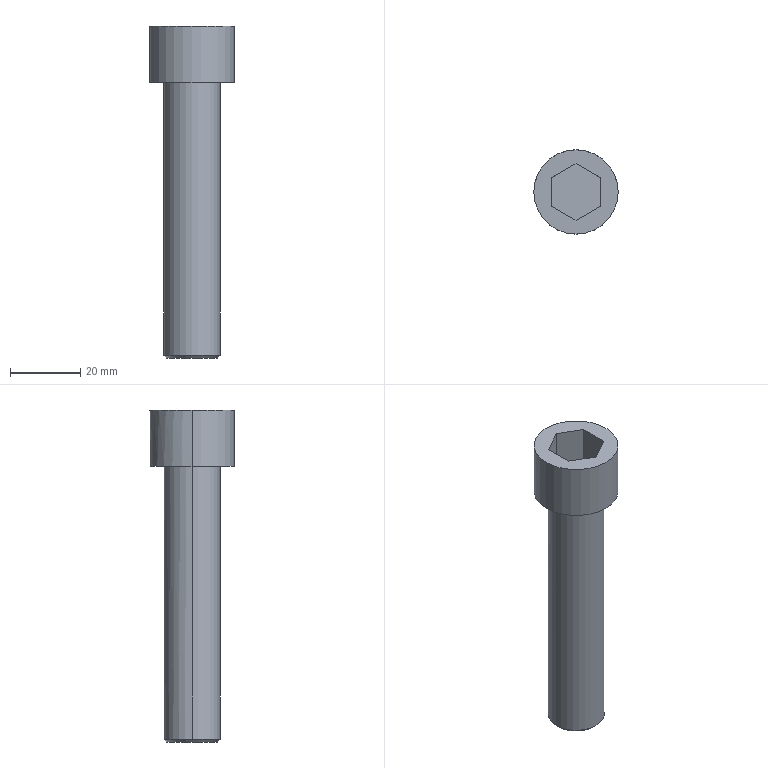Part | Creo | 1 solid | 16 faces | box 24 x 24 x 94.5 mm | volume 21213 mm3 | plane 10 | cylinder 4 | cone 2 | commonest cylinder face diameters 16 x2 24 x2
STEP:
#1=CARTESIAN_POINT('',(0.,0.,0.));
#2=DIRECTION('',(0.,0.,1.));
#3=DIRECTION('',(1.,0.,0.));
#4=AXIS2_PLACEMENT_3D('',#1,#2,#3);
#5=CARTESIAN_POINT('',(271.101,85.373,96.87));
#6=VERTEX_POINT('',#5);
#7=CARTESIAN_POINT('',(287.101,85.373,96.87));
#8=VERTEX_POINT('',#7);
#9=CARTESIAN_POINT('',(279.101,85.373,96.87));
#10=DIRECTION('',(0.,0.,-1.));
#11=DIRECTION('',(-1.,0.,0.));
#12=AXIS2_PLACEMENT_3D('',#9,#10,#11);
#13=CIRCLE('',#12,8.);
#14=EDGE_CURVE('',#6,#8,#13,.T.);
#15=ORIENTED_EDGE('',*,*,#14,.T.);
#16=CARTESIAN_POINT('',(287.101,85.373,174.559));
#17=VERTEX_POINT('',#16);
#18=CARTESIAN_POINT('',(287.101,85.373,174.559));
#19=DIRECTION('',(0.,0.,-1.));
#20=VECTOR('',#19,77.688);
#21=LINE('',#18,#20);
#22=EDGE_CURVE('',#17,#8,#21,.T.);
#23=ORIENTED_EDGE('',*,*,#22,.F.);
#24=CARTESIAN_POINT('',(279.101,93.373,174.559));
#25=VERTEX_POINT('',#24);
#26=CARTESIAN_POINT('',(279.101,85.373,174.559));
#27=DIRECTION('',(0.,0.,1.));
#28=DIRECTION('',(1.,0.,0.));
#29=AXIS2_PLACEMENT_3D('',#26,#27,#28);
#30=CIRCLE('',#29,8.);
#31=EDGE_CURVE('',#17,#25,#30,.T.);
#32=ORIENTED_EDGE('',*,*,#31,.T.);
#33=CARTESIAN_POINT('',(271.101,85.373,174.559));
#34=VERTEX_POINT('',#33);
#35=CARTESIAN_POINT('',(279.101,85.373,174.559));
#36=DIRECTION('',(0.,0.,1.));
#37=DIRECTION('',(0.,1.,0.));
#38=AXIS2_PLACEMENT_3D('',#35,#36,#37);
#39=CIRCLE('',#38,8.);
#40=EDGE_CURVE('',#25,#34,#39,.T.);
#41=ORIENTED_EDGE('',*,*,#40,.T.);
#42=CARTESIAN_POINT('',(271.101,85.373,174.559));
#43=DIRECTION('',(0.,0.,-1.));
#44=VECTOR('',#43,77.688);
#45=LINE('',#42,#44);
#46=EDGE_CURVE('',#34,#6,#45,.T.);
#47=ORIENTED_EDGE('',*,*,#46,.T.);
#48=EDGE_LOOP('',(#15,#23,#32,#41,#47));
#49=FACE_OUTER_BOUND('',#48,.F.);
#50=CARTESIAN_POINT('',(279.101,85.373,174.559));
#51=DIRECTION('',(0.,0.,-1.));
#52=DIRECTION('',(-1.,0.,0.));
#53=AXIS2_PLACEMENT_3D('',#50,#51,#52);
#54=CYLINDRICAL_SURFACE('',#53,8.);
#55=ADVANCED_FACE('',(#49),#54,.T.);
#56=CARTESIAN_POINT('',(279.101,92.561,96.059));
#57=VERTEX_POINT('',#56);
#58=CARTESIAN_POINT('',(286.289,85.373,96.059));
#59=VERTEX_POINT('',#58);
#60=CARTESIAN_POINT('',(279.101,85.373,96.059));
#61=DIRECTION('',(0.,0.,-1.));
#62=DIRECTION('',(0.,1.,0.));
#63=AXIS2_PLACEMENT_3D('',#60,#61,#62);
#64=CIRCLE('',#63,7.188);
#65=EDGE_CURVE('',#57,#59,#64,.T.);
#66=ORIENTED_EDGE('',*,*,#65,.T.);
#67=CARTESIAN_POINT('',(286.289,85.373,96.059));
#68=DIRECTION('',(0.7071,0.,0.7071));
#69=VECTOR('',#68,1.148);
#70=LINE('',#67,#69);
#71=EDGE_CURVE('',#59,#8,#70,.T.);
#72=ORIENTED_EDGE('',*,*,#71,.T.);
#73=ORIENTED_EDGE('',*,*,#14,.F.);
#74=CARTESIAN_POINT('',(271.913,85.373,96.059));
#75=VERTEX_POINT('',#74);
#76=CARTESIAN_POINT('',(271.913,85.373,96.059));
#77=DIRECTION('',(-0.7071,0.,0.7071));
#78=VECTOR('',#77,1.148);
#79=LINE('',#76,#78);
#80=EDGE_CURVE('',#75,#6,#79,.T.);
#81=ORIENTED_EDGE('',*,*,#80,.F.);
#82=CARTESIAN_POINT('',(279.101,85.373,96.059));
#83=DIRECTION('',(0.,0.,-1.));
#84=DIRECTION('',(-1.,0.,0.));
#85=AXIS2_PLACEMENT_3D('',#82,#83,#84);
#86=CIRCLE('',#85,7.188);
#87=EDGE_CURVE('',#75,#57,#86,.T.);
#88=ORIENTED_EDGE('',*,*,#87,.T.);
#89=EDGE_LOOP('',(#66,#72,#73,#81,#88));
#90=FACE_OUTER_BOUND('',#89,.F.);
#91=CARTESIAN_POINT('',(279.101,85.373,96.464));
#92=DIRECTION('',(0.,0.,1.));
#93=DIRECTION('',(1.,0.,0.));
#94=AXIS2_PLACEMENT_3D('',#91,#92,#93);
#95=CONICAL_SURFACE('',#94,7.594,45.);
#96=ADVANCED_FACE('',(#90),#95,.T.);
#97=CARTESIAN_POINT('',(279.101,78.184,96.059));
#98=VERTEX_POINT('',#97);
#99=CARTESIAN_POINT('',(279.101,85.373,96.059));
#100=DIRECTION('',(0.,0.,-1.));
#101=DIRECTION('',(0.,-1.,0.));
#102=AXIS2_PLACEMENT_3D('',#99,#100,#101);
#103=CIRCLE('',#102,7.188);
#104=EDGE_CURVE('',#98,#75,#103,.T.);
#105=ORIENTED_EDGE('',*,*,#104,.F.);
#106=CARTESIAN_POINT('',(279.101,85.373,96.059));
#107=DIRECTION('',(0.,0.,-1.));
#108=DIRECTION('',(1.,0.,0.));
#109=AXIS2_PLACEMENT_3D('',#106,#107,#108);
#110=CIRCLE('',#109,7.188);
#111=EDGE_CURVE('',#59,#98,#110,.T.);
#112=ORIENTED_EDGE('',*,*,#111,.F.);
#113=ORIENTED_EDGE('',*,*,#65,.F.);
#114=ORIENTED_EDGE('',*,*,#87,.F.);
#115=EDGE_LOOP('',(#105,#112,#113,#114));
#116=FACE_OUTER_BOUND('',#115,.F.);
#117=CARTESIAN_POINT('',(279.101,85.373,96.059));
#118=DIRECTION('',(0.,0.,1.));
#119=DIRECTION('',(1.,0.,0.));
#120=AXIS2_PLACEMENT_3D('',#117,#118,#119);
#121=PLANE('',#120);
#122=ADVANCED_FACE('',(#116),#121,.F.);
#123=ORIENTED_EDGE('',*,*,#111,.T.);
#124=ORIENTED_EDGE('',*,*,#104,.T.);
#125=ORIENTED_EDGE('',*,*,#80,.T.);
#126=CARTESIAN_POINT('',(279.101,77.373,96.87));
#127=VERTEX_POINT('',#126);
#128=CARTESIAN_POINT('',(279.101,85.373,96.87));
#129=DIRECTION('',(0.,0.,-1.));
#130=DIRECTION('',(0.,-1.,0.));
#131=AXIS2_PLACEMENT_3D('',#128,#129,#130);
#132=CIRCLE('',#131,8.);
#133=EDGE_CURVE('',#127,#6,#132,.T.);
#134=ORIENTED_EDGE('',*,*,#133,.F.);
#135=CARTESIAN_POINT('',(279.101,85.373,96.87));
#136=DIRECTION('',(0.,0.,-1.));
#137=DIRECTION('',(1.,0.,0.));
#138=AXIS2_PLACEMENT_3D('',#135,#136,#137);
#139=CIRCLE('',#138,8.);
#140=EDGE_CURVE('',#8,#127,#139,.T.);
#141=ORIENTED_EDGE('',*,*,#140,.F.);
#142=ORIENTED_EDGE('',*,*,#71,.F.);
#143=EDGE_LOOP('',(#123,#124,#125,#134,#141,#142));
#144=FACE_OUTER_BOUND('',#143,.F.);
#145=CARTESIAN_POINT('',(279.101,85.373,96.464));
#146=DIRECTION('',(0.,0.,1.));
#147=DIRECTION('',(1.,0.,0.));
#148=AXIS2_PLACEMENT_3D('',#145,#146,#147);
#149=CONICAL_SURFACE('',#148,7.594,45.);
#150=ADVANCED_FACE('',(#144),#149,.T.);
#151=ORIENTED_EDGE('',*,*,#140,.T.);
#152=ORIENTED_EDGE('',*,*,#133,.T.);
#153=ORIENTED_EDGE('',*,*,#46,.F.);
#154=CARTESIAN_POINT('',(279.101,77.373,174.559));
#155=VERTEX_POINT('',#154);
#156=CARTESIAN_POINT('',(279.101,85.373,174.559));
#157=DIRECTION('',(0.,0.,1.));
#158=DIRECTION('',(-1.,0.,0.));
#159=AXIS2_PLACEMENT_3D('',#156,#157,#158);
#160=CIRCLE('',#159,8.);
#161=EDGE_CURVE('',#34,#155,#160,.T.);
#162=ORIENTED_EDGE('',*,*,#161,.T.);
#163=CARTESIAN_POINT('',(279.101,85.373,174.559));
#164=DIRECTION('',(0.,0.,1.));
#165=DIRECTION('',(0.,-1.,0.));
#166=AXIS2_PLACEMENT_3D('',#163,#164,#165);
#167=CIRCLE('',#166,8.);
#168=EDGE_CURVE('',#155,#17,#167,.T.);
#169=ORIENTED_EDGE('',*,*,#168,.T.);
#170=ORIENTED_EDGE('',*,*,#22,.T.);
#171=EDGE_LOOP('',(#151,#152,#153,#162,#169,#170));
#172=FACE_OUTER_BOUND('',#171,.F.);
#173=CARTESIAN_POINT('',(279.101,85.373,174.559));
#174=DIRECTION('',(0.,0.,-1.));
#175=DIRECTION('',(-1.,0.,0.));
#176=AXIS2_PLACEMENT_3D('',#173,#174,#175);
#177=CYLINDRICAL_SURFACE('',#176,8.);
#178=ADVANCED_FACE('',(#172),#177,.T.);
#179=CARTESIAN_POINT('',(279.101,73.373,174.559));
#180=VERTEX_POINT('',#179);
#181=CARTESIAN_POINT('',(267.101,85.373,174.559));
#182=VERTEX_POINT('',#181);
#183=CARTESIAN_POINT('',(279.101,85.373,174.559));
#184=DIRECTION('',(0.,0.,-1.));
#185=DIRECTION('',(0.,-1.,0.));
#186=AXIS2_PLACEMENT_3D('',#183,#184,#185);
#187=CIRCLE('',#186,12.);
#188=EDGE_CURVE('',#180,#182,#187,.T.);
#189=ORIENTED_EDGE('',*,*,#188,.F.);
#190=CARTESIAN_POINT('',(291.101,85.373,174.559));
#191=VERTEX_POINT('',#190);
#192=CARTESIAN_POINT('',(279.101,85.373,174.559));
#193=DIRECTION('',(0.,0.,-1.));
#194=DIRECTION('',(1.,0.,0.));
#195=AXIS2_PLACEMENT_3D('',#192,#193,#194);
#196=CIRCLE('',#195,12.);
#197=EDGE_CURVE('',#191,#180,#196,.T.);
#198=ORIENTED_EDGE('',*,*,#197,.F.);
#199=CARTESIAN_POINT('',(279.101,85.373,174.559));
#200=DIRECTION('',(0.,0.,-1.));
#201=DIRECTION('',(-1.,0.,0.));
#202=AXIS2_PLACEMENT_3D('',#199,#200,#201);
#203=CIRCLE('',#202,12.);
#204=EDGE_CURVE('',#182,#191,#203,.T.);
#205=ORIENTED_EDGE('',*,*,#204,.F.);
#206=EDGE_LOOP('',(#189,#198,#205));
#207=FACE_OUTER_BOUND('',#206,.F.);
#208=ORIENTED_EDGE('',*,*,#168,.F.);
#209=ORIENTED_EDGE('',*,*,#161,.F.);
#210=ORIENTED_EDGE('',*,*,#40,.F.);
#211=ORIENTED_EDGE('',*,*,#31,.F.);
#212=EDGE_LOOP('',(#208,#209,#210,#211));
#213=FACE_BOUND('',#212,.F.);
#214=CARTESIAN_POINT('',(279.101,85.373,174.559));
#215=DIRECTION('',(0.,0.,-1.));
#216=DIRECTION('',(-1.,0.,0.));
#217=AXIS2_PLACEMENT_3D('',#214,#215,#216);
#218=PLANE('',#217);
#219=ADVANCED_FACE('',(#207,#213),#218,.T.);
#220=CARTESIAN_POINT('',(267.101,85.373,190.559));
#221=VERTEX_POINT('',#220);
#222=CARTESIAN_POINT('',(279.101,73.373,190.559));
#223=VERTEX_POINT('',#222);
#224=CARTESIAN_POINT('',(279.101,85.373,190.559));
#225=DIRECTION('',(0.,0.,1.));
#226=DIRECTION('',(-1.,0.,0.));
#227=AXIS2_PLACEMENT_3D('',#224,#225,#226);
#228=CIRCLE('',#227,12.);
#229=EDGE_CURVE('',#221,#223,#228,.T.);
#230=ORIENTED_EDGE('',*,*,#229,.T.);
#231=CARTESIAN_POINT('',(291.101,85.373,190.559));
#232=VERTEX_POINT('',#231);
#233=CARTESIAN_POINT('',(279.101,85.373,190.559));
#234=DIRECTION('',(0.,0.,1.));
#235=DIRECTION('',(0.,-1.,0.));
#236=AXIS2_PLACEMENT_3D('',#233,#234,#235);
#237=CIRCLE('',#236,12.);
#238=EDGE_CURVE('',#223,#232,#237,.T.);
#239=ORIENTED_EDGE('',*,*,#238,.T.);
#240=CARTESIAN_POINT('',(291.101,85.373,174.559));
#241=DIRECTION('',(0.,0.,1.));
#242=VECTOR('',#241,16.);
#243=LINE('',#240,#242);
#244=EDGE_CURVE('',#191,#232,#243,.T.);
#245=ORIENTED_EDGE('',*,*,#244,.F.);
#246=ORIENTED_EDGE('',*,*,#197,.T.);
#247=ORIENTED_EDGE('',*,*,#188,.T.);
#248=CARTESIAN_POINT('',(267.101,85.373,174.559));
#249=DIRECTION('',(0.,0.,1.));
#250=VECTOR('',#249,16.);
#251=LINE('',#248,#250);
#252=EDGE_CURVE('',#182,#221,#251,.T.);
#253=ORIENTED_EDGE('',*,*,#252,.T.);
#254=EDGE_LOOP('',(#230,#239,#245,#246,#247,#253));
#255=FACE_OUTER_BOUND('',#254,.F.);
#256=CARTESIAN_POINT('',(279.101,85.373,174.559));
#257=DIRECTION('',(0.,0.,1.));
#258=DIRECTION('',(1.,0.,0.));
#259=AXIS2_PLACEMENT_3D('',#256,#257,#258);
#260=CYLINDRICAL_SURFACE('',#259,12.);
#261=ADVANCED_FACE('',(#255),#260,.T.);
#262=ORIENTED_EDGE('',*,*,#238,.F.);
#263=ORIENTED_EDGE('',*,*,#229,.F.);
#264=CARTESIAN_POINT('',(279.101,97.373,190.559));
#265=VERTEX_POINT('',#264);
#266=CARTESIAN_POINT('',(279.101,85.373,190.559));
#267=DIRECTION('',(0.,0.,1.));
#268=DIRECTION('',(0.,1.,0.));
#269=AXIS2_PLACEMENT_3D('',#266,#267,#268);
#270=CIRCLE('',#269,12.);
#271=EDGE_CURVE('',#265,#221,#270,.T.);
#272=ORIENTED_EDGE('',*,*,#271,.F.);
#273=CARTESIAN_POINT('',(279.101,85.373,190.559));
#274=DIRECTION('',(0.,0.,1.));
#275=DIRECTION('',(1.,0.,0.));
#276=AXIS2_PLACEMENT_3D('',#273,#274,#275);
#277=CIRCLE('',#276,12.);
#278=EDGE_CURVE('',#232,#265,#277,.T.);
#279=ORIENTED_EDGE('',*,*,#278,.F.);
#280=EDGE_LOOP('',(#262,#263,#272,#279));
#281=FACE_OUTER_BOUND('',#280,.F.);
#282=CARTESIAN_POINT('',(272.101,81.331,190.559));
#283=VERTEX_POINT('',#282);
#284=CARTESIAN_POINT('',(272.101,89.414,190.559));
#285=VERTEX_POINT('',#284);
#286=CARTESIAN_POINT('',(272.101,81.331,190.559));
#287=DIRECTION('',(0.,1.,0.));
#288=VECTOR('',#287,8.083);
#289=LINE('',#286,#288);
#290=EDGE_CURVE('',#283,#285,#289,.T.);
#291=ORIENTED_EDGE('',*,*,#290,.F.);
#292=CARTESIAN_POINT('',(279.101,77.29,190.559));
#293=VERTEX_POINT('',#292);
#294=CARTESIAN_POINT('',(279.101,77.29,190.559));
#295=DIRECTION('',(-0.866,0.5,0.));
#296=VECTOR('',#295,8.083);
#297=LINE('',#294,#296);
#298=EDGE_CURVE('',#293,#283,#297,.T.);
#299=ORIENTED_EDGE('',*,*,#298,.F.);
#300=CARTESIAN_POINT('',(286.101,81.331,190.559));
#301=VERTEX_POINT('',#300);
#302=CARTESIAN_POINT('',(286.101,81.331,190.559));
#303=DIRECTION('',(-0.866,-0.5,0.));
#304=VECTOR('',#303,8.083);
#305=LINE('',#302,#304);
#306=EDGE_CURVE('',#301,#293,#305,.T.);
#307=ORIENTED_EDGE('',*,*,#306,.F.);
#308=CARTESIAN_POINT('',(286.101,89.414,190.559));
#309=VERTEX_POINT('',#308);
#310=CARTESIAN_POINT('',(286.101,89.414,190.559));
#311=DIRECTION('',(0.,-1.,0.));
#312=VECTOR('',#311,8.083);
#313=LINE('',#310,#312);
#314=EDGE_CURVE('',#309,#301,#313,.T.);
#315=ORIENTED_EDGE('',*,*,#314,.F.);
#316=CARTESIAN_POINT('',(279.101,93.455,190.559));
#317=VERTEX_POINT('',#316);
#318=CARTESIAN_POINT('',(279.101,93.455,190.559));
#319=DIRECTION('',(0.866,-0.5,0.));
#320=VECTOR('',#319,8.083);
#321=LINE('',#318,#320);
#322=EDGE_CURVE('',#317,#309,#321,.T.);
#323=ORIENTED_EDGE('',*,*,#322,.F.);
#324=CARTESIAN_POINT('',(272.101,89.414,190.559));
#325=DIRECTION('',(0.866,0.5,0.));
#326=VECTOR('',#325,8.083);
#327=LINE('',#324,#326);
#328=EDGE_CURVE('',#285,#317,#327,.T.);
#329=ORIENTED_EDGE('',*,*,#328,.F.);
#330=EDGE_LOOP('',(#291,#299,#307,#315,#323,#329));
#331=FACE_BOUND('',#330,.F.);
#332=CARTESIAN_POINT('',(279.101,85.373,190.559));
#333=DIRECTION('',(0.,0.,1.));
#334=DIRECTION('',(1.,0.,0.));
#335=AXIS2_PLACEMENT_3D('',#332,#333,#334);
#336=PLANE('',#335);
#337=ADVANCED_FACE('',(#281,#331),#336,.T.);
#338=ORIENTED_EDGE('',*,*,#290,.T.);
#339=CARTESIAN_POINT('',(272.101,89.414,179.999));
#340=VERTEX_POINT('',#339);
#341=CARTESIAN_POINT('',(272.101,89.414,190.559));
#342=DIRECTION('',(0.,0.,-1.));
#343=VECTOR('',#342,10.56);
#344=LINE('',#341,#343);
#345=EDGE_CURVE('',#285,#340,#344,.T.);
#346=ORIENTED_EDGE('',*,*,#345,.T.);
#347=CARTESIAN_POINT('',(272.101,81.331,179.999));
#348=VERTEX_POINT('',#347);
#349=CARTESIAN_POINT('',(272.101,81.331,179.999));
#350=DIRECTION('',(0.,1.,0.));
#351=VECTOR('',#350,8.083);
#352=LINE('',#349,#351);
#353=EDGE_CURVE('',#348,#340,#352,.T.);
#354=ORIENTED_EDGE('',*,*,#353,.F.);
#355=CARTESIAN_POINT('',(272.101,81.331,190.559));
#356=DIRECTION('',(0.,0.,-1.));
#357=VECTOR('',#356,10.56);
#358=LINE('',#355,#357);
#359=EDGE_CURVE('',#283,#348,#358,.T.);
#360=ORIENTED_EDGE('',*,*,#359,.F.);
#361=EDGE_LOOP('',(#338,#346,#354,#360));
#362=FACE_OUTER_BOUND('',#361,.F.);
#363=CARTESIAN_POINT('',(272.101,89.414,179.999));
#364=DIRECTION('',(-1.,0.,0.));
#365=DIRECTION('',(0.,0.,1.));
#366=AXIS2_PLACEMENT_3D('',#363,#364,#365);
#367=PLANE('',#366);
#368=ADVANCED_FACE('',(#362),#367,.F.);
#369=ORIENTED_EDGE('',*,*,#328,.T.);
#370=CARTESIAN_POINT('',(279.101,93.455,179.999));
#371=VERTEX_POINT('',#370);
#372=CARTESIAN_POINT('',(279.101,93.455,190.559));
#373=DIRECTION('',(0.,0.,-1.));
#374=VECTOR('',#373,10.56);
#375=LINE('',#372,#374);
#376=EDGE_CURVE('',#317,#371,#375,.T.);
#377=ORIENTED_EDGE('',*,*,#376,.T.);
#378=CARTESIAN_POINT('',(279.101,93.455,179.999));
#379=DIRECTION('',(-0.866,-0.5,0.));
#380=VECTOR('',#379,8.083);
#381=LINE('',#378,#380);
#382=EDGE_CURVE('',#371,#340,#381,.T.);
#383=ORIENTED_EDGE('',*,*,#382,.T.);
#384=ORIENTED_EDGE('',*,*,#345,.F.);
#385=EDGE_LOOP('',(#369,#377,#383,#384));
#386=FACE_OUTER_BOUND('',#385,.F.);
#387=CARTESIAN_POINT('',(279.101,93.455,179.999));
#388=DIRECTION('',(-0.5,0.866,0.));
#389=DIRECTION('',(-0.866,-0.5,0.));
#390=AXIS2_PLACEMENT_3D('',#387,#388,#389);
#391=PLANE('',#390);
#392=ADVANCED_FACE('',(#386),#391,.F.);
#393=ORIENTED_EDGE('',*,*,#322,.T.);
#394=CARTESIAN_POINT('',(286.101,89.414,179.999));
#395=VERTEX_POINT('',#394);
#396=CARTESIAN_POINT('',(286.101,89.414,190.559));
#397=DIRECTION('',(0.,0.,-1.));
#398=VECTOR('',#397,10.56);
#399=LINE('',#396,#398);
#400=EDGE_CURVE('',#309,#395,#399,.T.);
#401=ORIENTED_EDGE('',*,*,#400,.T.);
#402=CARTESIAN_POINT('',(286.101,89.414,179.999));
#403=DIRECTION('',(-0.866,0.5,0.));
#404=VECTOR('',#403,8.083);
#405=LINE('',#402,#404);
#406=EDGE_CURVE('',#395,#371,#405,.T.);
#407=ORIENTED_EDGE('',*,*,#406,.T.);
#408=ORIENTED_EDGE('',*,*,#376,.F.);
#409=EDGE_LOOP('',(#393,#401,#407,#408));
#410=FACE_OUTER_BOUND('',#409,.F.);
#411=CARTESIAN_POINT('',(286.101,89.414,179.999));
#412=DIRECTION('',(0.5,0.866,0.));
#413=DIRECTION('',(-0.866,0.5,0.));
#414=AXIS2_PLACEMENT_3D('',#411,#412,#413);
#415=PLANE('',#414);
#416=ADVANCED_FACE('',(#410),#415,.F.);
#417=ORIENTED_EDGE('',*,*,#314,.T.);
#418=CARTESIAN_POINT('',(286.101,81.331,179.999));
#419=VERTEX_POINT('',#418);
#420=CARTESIAN_POINT('',(286.101,81.331,190.559));
#421=DIRECTION('',(0.,0.,-1.));
#422=VECTOR('',#421,10.56);
#423=LINE('',#420,#422);
#424=EDGE_CURVE('',#301,#419,#423,.T.);
#425=ORIENTED_EDGE('',*,*,#424,.T.);
#426=CARTESIAN_POINT('',(286.101,89.414,179.999));
#427=DIRECTION('',(0.,-1.,0.));
#428=VECTOR('',#427,8.083);
#429=LINE('',#426,#428);
#430=EDGE_CURVE('',#395,#419,#429,.T.);
#431=ORIENTED_EDGE('',*,*,#430,.F.);
#432=ORIENTED_EDGE('',*,*,#400,.F.);
#433=EDGE_LOOP('',(#417,#425,#431,#432));
#434=FACE_OUTER_BOUND('',#433,.F.);
#435=CARTESIAN_POINT('',(286.101,81.331,179.999));
#436=DIRECTION('',(1.,0.,0.));
#437=DIRECTION('',(0.,0.,-1.));
#438=AXIS2_PLACEMENT_3D('',#435,#436,#437);
#439=PLANE('',#438);
#440=ADVANCED_FACE('',(#434),#439,.F.);
#441=ORIENTED_EDGE('',*,*,#306,.T.);
#442=CARTESIAN_POINT('',(279.101,77.29,179.999));
#443=VERTEX_POINT('',#442);
#444=CARTESIAN_POINT('',(279.101,77.29,190.559));
#445=DIRECTION('',(0.,0.,-1.));
#446=VECTOR('',#445,10.56);
#447=LINE('',#444,#446);
#448=EDGE_CURVE('',#293,#443,#447,.T.);
#449=ORIENTED_EDGE('',*,*,#448,.T.);
#450=CARTESIAN_POINT('',(279.101,77.29,179.999));
#451=DIRECTION('',(0.866,0.5,0.));
#452=VECTOR('',#451,8.083);
#453=LINE('',#450,#452);
#454=EDGE_CURVE('',#443,#419,#453,.T.);
#455=ORIENTED_EDGE('',*,*,#454,.T.);
#456=ORIENTED_EDGE('',*,*,#424,.F.);
#457=EDGE_LOOP('',(#441,#449,#455,#456));
#458=FACE_OUTER_BOUND('',#457,.F.);
#459=CARTESIAN_POINT('',(279.101,77.29,179.999));
#460=DIRECTION('',(0.5,-0.866,0.));
#461=DIRECTION('',(0.866,0.5,0.));
#462=AXIS2_PLACEMENT_3D('',#459,#460,#461);
#463=PLANE('',#462);
#464=ADVANCED_FACE('',(#458),#463,.F.);
#465=ORIENTED_EDGE('',*,*,#298,.T.);
#466=ORIENTED_EDGE('',*,*,#359,.T.);
#467=CARTESIAN_POINT('',(272.101,81.331,179.999));
#468=DIRECTION('',(0.866,-0.5,0.));
#469=VECTOR('',#468,8.083);
#470=LINE('',#467,#469);
#471=EDGE_CURVE('',#348,#443,#470,.T.);
#472=ORIENTED_EDGE('',*,*,#471,.T.);
#473=ORIENTED_EDGE('',*,*,#448,.F.);
#474=EDGE_LOOP('',(#465,#466,#472,#473));
#475=FACE_OUTER_BOUND('',#474,.F.);
#476=CARTESIAN_POINT('',(272.101,81.331,179.999));
#477=DIRECTION('',(-0.5,-0.866,0.));
#478=DIRECTION('',(0.866,-0.5,0.));
#479=AXIS2_PLACEMENT_3D('',#476,#477,#478);
#480=PLANE('',#479);
#481=ADVANCED_FACE('',(#475),#480,.F.);
#482=ORIENTED_EDGE('',*,*,#353,.T.);
#483=ORIENTED_EDGE('',*,*,#382,.F.);
#484=ORIENTED_EDGE('',*,*,#406,.F.);
#485=ORIENTED_EDGE('',*,*,#430,.T.);
#486=ORIENTED_EDGE('',*,*,#454,.F.);
#487=ORIENTED_EDGE('',*,*,#471,.F.);
#488=EDGE_LOOP('',(#482,#483,#484,#485,#486,#487));
#489=FACE_OUTER_BOUND('',#488,.F.);
#490=CARTESIAN_POINT('',(272.101,81.331,179.999));
#491=DIRECTION('',(0.,0.,1.));
#492=DIRECTION('',(1.,0.,0.));
#493=AXIS2_PLACEMENT_3D('',#490,#491,#492);
#494=PLANE('',#493);
#495=ADVANCED_FACE('',(#489),#494,.T.);
#496=ORIENTED_EDGE('',*,*,#271,.T.);
#497=ORIENTED_EDGE('',*,*,#252,.F.);
#498=ORIENTED_EDGE('',*,*,#204,.T.);
#499=ORIENTED_EDGE('',*,*,#244,.T.);
#500=ORIENTED_EDGE('',*,*,#278,.T.);
#501=EDGE_LOOP('',(#496,#497,#498,#499,#500));
#502=FACE_OUTER_BOUND('',#501,.F.);
#503=CARTESIAN_POINT('',(279.101,85.373,174.559));
#504=DIRECTION('',(0.,0.,1.));
#505=DIRECTION('',(1.,0.,0.));
#506=AXIS2_PLACEMENT_3D('',#503,#504,#505);
#507=CYLINDRICAL_SURFACE('',#506,12.);
#508=ADVANCED_FACE('',(#502),#507,.T.);
#509=CLOSED_SHELL('',(#55,#96,#122,#150,#178,#219,#261,#337,#368,#392,#416,#440,#464,#481,#495,#508));
#510=MANIFOLD_SOLID_BREP('',#509);
#511=(LENGTH_UNIT()NAMED_UNIT(*)SI_UNIT(.MILLI.,.METRE.));
#512=UNCERTAINTY_MEASURE_WITH_UNIT(LENGTH_MEASURE(0.01004),#511,'','');
#513=(NAMED_UNIT(*)PLANE_ANGLE_UNIT()SI_UNIT($,.RADIAN.));
#514=PLANE_ANGLE_MEASURE_WITH_UNIT(PLANE_ANGLE_MEASURE(0.01745),#513);
#515=(CONVERSION_BASED_UNIT('DEGREE',#514)NAMED_UNIT(*)PLANE_ANGLE_UNIT());
#516=(NAMED_UNIT(*)SI_UNIT($,.STERADIAN.)SOLID_ANGLE_UNIT());
#517=(GEOMETRIC_REPRESENTATION_CONTEXT(3)GLOBAL_UNCERTAINTY_ASSIGNED_CONTEXT((#512))GLOBAL_UNIT_ASSIGNED_CONTEXT((#511,#515,#516))REPRESENTATION_CONTEXT('',''));
#518=ADVANCED_BREP_SHAPE_REPRESENTATION('',(#4,#510),#517);